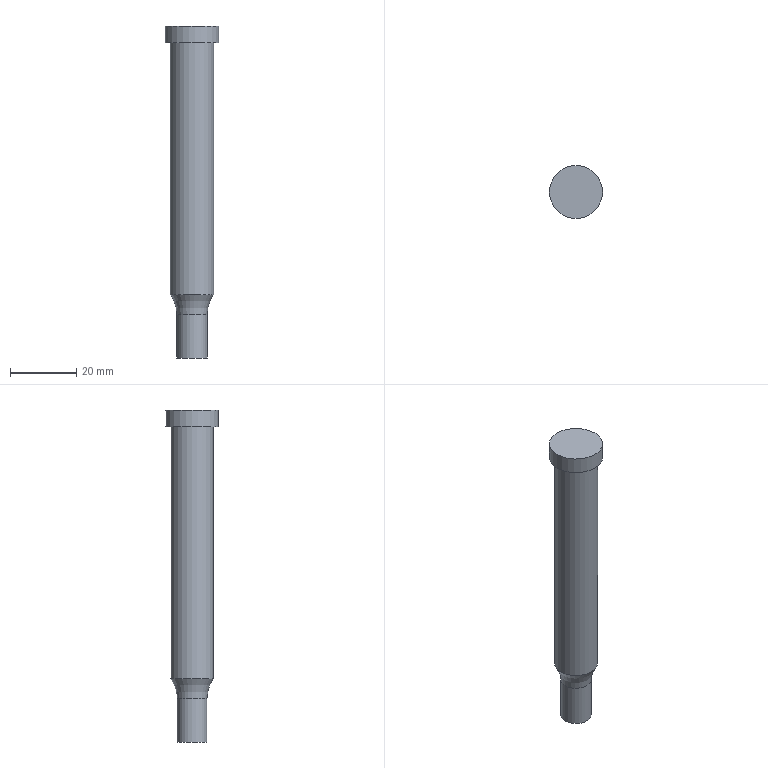Part | NX | features SPAS 13-80-10.10 2 | 1 solid | 7 faces | box 16 x 16 x 100 mm | volume 12445 mm3 | plane 3 | cylinder 3 | torus 1 | commonest cylinder face diameters 9.1 x1 13 x1 16 x1
STEP:
#1=CARTESIAN_POINT('',(771.01,-1.948,11.));
#2=VERTEX_POINT('',#1);
#3=CARTESIAN_POINT('',(775.56,-1.948,11.));
#4=DIRECTION('',(0.,0.,-1.));
#5=DIRECTION('',(-1.,0.,0.));
#6=AXIS2_PLACEMENT_3D('',#3,#4,#5);
#7=CIRCLE('',#6,4.55);
#8=EDGE_CURVE('',#2,#2,#7,.F.);
#9=ORIENTED_EDGE('',*,*,#8,.F.);
#10=EDGE_LOOP('',(#9));
#11=FACE_BOUND('',#10,.T.);
#12=CARTESIAN_POINT('',(775.56,-1.948,11.));
#13=DIRECTION('',(0.,0.,-1.));
#14=DIRECTION('',(-1.,0.,0.));
#15=AXIS2_PLACEMENT_3D('',#12,#13,#14);
#16=PLANE('',#15);
#17=ADVANCED_FACE('',(#11),#16,.T.);
#18=CARTESIAN_POINT('',(780.11,-1.948,24.));
#19=VERTEX_POINT('',#18);
#20=CARTESIAN_POINT('',(775.56,-1.948,24.));
#21=DIRECTION('',(0.,0.,1.));
#22=DIRECTION('',(1.,0.,0.));
#23=AXIS2_PLACEMENT_3D('',#20,#21,#22);
#24=CIRCLE('',#23,4.55);
#25=EDGE_CURVE('',#19,#19,#24,.F.);
#26=ORIENTED_EDGE('',*,*,#25,.T.);
#27=EDGE_LOOP('',(#26));
#28=FACE_BOUND('',#27,.T.);
#29=ORIENTED_EDGE('',*,*,#8,.T.);
#30=EDGE_LOOP('',(#29));
#31=FACE_BOUND('',#30,.T.);
#32=CARTESIAN_POINT('',(775.56,-1.948,11.));
#33=DIRECTION('',(0.,0.,1.));
#34=DIRECTION('',(1.,0.,0.));
#35=AXIS2_PLACEMENT_3D('',#32,#33,#34);
#36=CYLINDRICAL_SURFACE('',#35,4.55);
#37=ADVANCED_FACE('',(#28,#31),#36,.T.);
#38=CARTESIAN_POINT('',(769.06,-1.948,106.));
#39=VERTEX_POINT('',#38);
#40=CARTESIAN_POINT('',(775.56,-1.948,106.));
#41=DIRECTION('',(0.,0.,-1.));
#42=DIRECTION('',(-1.,0.,0.));
#43=AXIS2_PLACEMENT_3D('',#40,#41,#42);
#44=CIRCLE('',#43,6.5);
#45=EDGE_CURVE('',#39,#39,#44,.F.);
#46=ORIENTED_EDGE('',*,*,#45,.F.);
#47=EDGE_LOOP('',(#46));
#48=FACE_BOUND('',#47,.T.);
#49=CARTESIAN_POINT('',(769.06,-1.948,30.095));
#50=VERTEX_POINT('',#49);
#51=CARTESIAN_POINT('',(775.56,-1.948,30.095));
#52=DIRECTION('',(0.,0.,-1.));
#53=DIRECTION('',(-1.,0.,0.));
#54=AXIS2_PLACEMENT_3D('',#51,#52,#53);
#55=CIRCLE('',#54,6.5);
#56=EDGE_CURVE('',#50,#50,#55,.F.);
#57=ORIENTED_EDGE('',*,*,#56,.T.);
#58=EDGE_LOOP('',(#57));
#59=FACE_BOUND('',#58,.T.);
#60=CARTESIAN_POINT('',(775.56,-1.948,29.186));
#61=DIRECTION('',(0.,0.,1.));
#62=DIRECTION('',(1.,0.,0.));
#63=AXIS2_PLACEMENT_3D('',#60,#61,#62);
#64=CYLINDRICAL_SURFACE('',#63,6.5);
#65=ADVANCED_FACE('',(#48,#59),#64,.T.);
#66=CARTESIAN_POINT('',(783.56,-1.948,111.));
#67=VERTEX_POINT('',#66);
#68=CARTESIAN_POINT('',(775.56,-1.948,111.));
#69=DIRECTION('',(0.,0.,1.));
#70=DIRECTION('',(1.,0.,0.));
#71=AXIS2_PLACEMENT_3D('',#68,#69,#70);
#72=CIRCLE('',#71,8.);
#73=EDGE_CURVE('',#67,#67,#72,.F.);
#74=ORIENTED_EDGE('',*,*,#73,.F.);
#75=EDGE_LOOP('',(#74));
#76=FACE_BOUND('',#75,.T.);
#77=CARTESIAN_POINT('',(775.56,-1.948,111.));
#78=DIRECTION('',(0.,0.,1.));
#79=DIRECTION('',(1.,0.,0.));
#80=AXIS2_PLACEMENT_3D('',#77,#78,#79);
#81=PLANE('',#80);
#82=ADVANCED_FACE('',(#76),#81,.T.);
#83=ORIENTED_EDGE('',*,*,#45,.T.);
#84=EDGE_LOOP('',(#83));
#85=FACE_BOUND('',#84,.T.);
#86=CARTESIAN_POINT('',(767.56,-1.948,106.));
#87=VERTEX_POINT('',#86);
#88=CARTESIAN_POINT('',(775.56,-1.948,106.));
#89=DIRECTION('',(0.,0.,-1.));
#90=DIRECTION('',(-1.,0.,0.));
#91=AXIS2_PLACEMENT_3D('',#88,#89,#90);
#92=CIRCLE('',#91,8.);
#93=EDGE_CURVE('',#87,#87,#92,.F.);
#94=ORIENTED_EDGE('',*,*,#93,.F.);
#95=EDGE_LOOP('',(#94));
#96=FACE_BOUND('',#95,.T.);
#97=CARTESIAN_POINT('',(775.56,-1.948,106.));
#98=DIRECTION('',(0.,0.,-1.));
#99=DIRECTION('',(-1.,0.,0.));
#100=AXIS2_PLACEMENT_3D('',#97,#98,#99);
#101=PLANE('',#100);
#102=ADVANCED_FACE('',(#85,#96),#101,.T.);
#103=ORIENTED_EDGE('',*,*,#73,.T.);
#104=EDGE_LOOP('',(#103));
#105=FACE_BOUND('',#104,.T.);
#106=ORIENTED_EDGE('',*,*,#93,.T.);
#107=EDGE_LOOP('',(#106));
#108=FACE_BOUND('',#107,.T.);
#109=CARTESIAN_POINT('',(775.56,-1.948,86.));
#110=DIRECTION('',(0.,0.,1.));
#111=DIRECTION('',(1.,0.,0.));
#112=AXIS2_PLACEMENT_3D('',#109,#110,#111);
#113=CYLINDRICAL_SURFACE('',#112,8.);
#114=ADVANCED_FACE('',(#105,#108),#113,.T.);
#115=ORIENTED_EDGE('',*,*,#25,.F.);
#116=EDGE_LOOP('',(#115));
#117=FACE_BOUND('',#116,.T.);
#118=ORIENTED_EDGE('',*,*,#56,.F.);
#119=EDGE_LOOP('',(#118));
#120=FACE_BOUND('',#119,.T.);
#121=CARTESIAN_POINT('',(775.56,-1.948,24.));
#122=DIRECTION('',(0.,0.,1.));
#123=DIRECTION('',(1.,0.,0.));
#124=AXIS2_PLACEMENT_3D('',#121,#122,#123);
#125=TOROIDAL_SURFACE('',#124,15.05,10.5);
#126=ADVANCED_FACE('',(#117,#120),#125,.F.);
#127=CLOSED_SHELL('',(#17,#37,#65,#82,#102,#114,#126));
#128=MANIFOLD_SOLID_BREP('',#127);
#129=(LENGTH_UNIT()NAMED_UNIT(*)SI_UNIT(.MILLI.,.METRE.));
#130=UNCERTAINTY_MEASURE_WITH_UNIT(LENGTH_MEASURE(0.00001),#129,'','');
#131=(NAMED_UNIT(*)PLANE_ANGLE_UNIT()SI_UNIT($,.RADIAN.));
#132=(NAMED_UNIT(*)SI_UNIT($,.STERADIAN.)SOLID_ANGLE_UNIT());
#133=(GEOMETRIC_REPRESENTATION_CONTEXT(3)GLOBAL_UNCERTAINTY_ASSIGNED_CONTEXT((#130))GLOBAL_UNIT_ASSIGNED_CONTEXT((#129,#131,#132))REPRESENTATION_CONTEXT('',''));
#134=ADVANCED_BREP_SHAPE_REPRESENTATION('',(#128),#133);